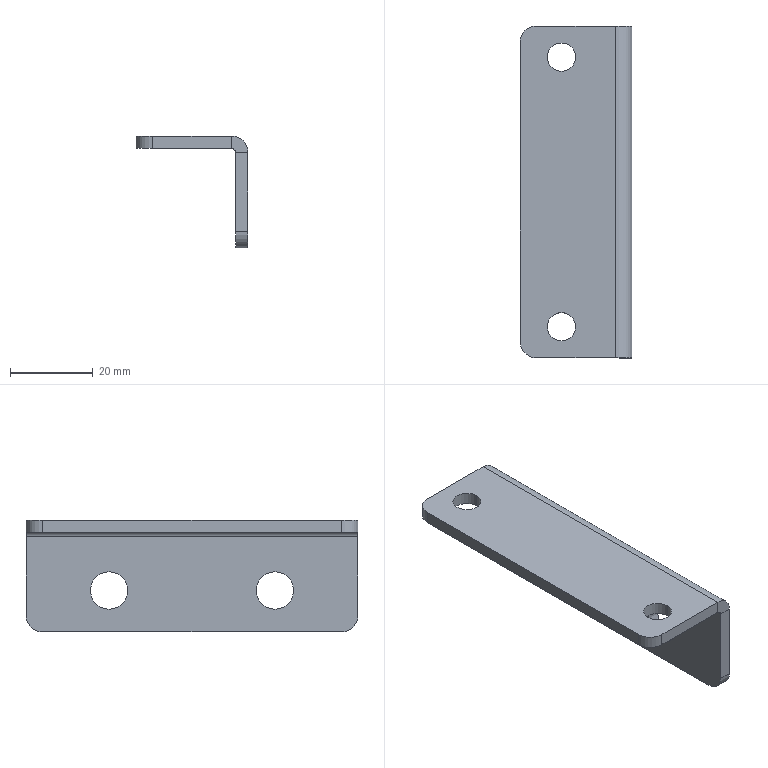Part | STEP file | 1.6米L型片 | 1 solid | 26 faces | box 27 x 80 x 27 mm | volume 11342 mm3 | cylinder 14 | plane 12 | commonest cylinder face diameters 8 x5 6.8 x4 9 x4 2 x1
STEP:
#1=CARTESIAN_POINT('',(27.,20.,-21.5));
#2=VERTEX_POINT('',#1);
#3=CARTESIAN_POINT('',(27.,20.,-12.5));
#4=VERTEX_POINT('',#3);
#5=CARTESIAN_POINT('',(27.,20.,-17.));
#6=DIRECTION('',(-1.,0.,0.));
#7=DIRECTION('',(0.,0.,1.));
#8=AXIS2_PLACEMENT_3D('',#5,#6,#7);
#9=CIRCLE('',#8,4.5);
#10=EDGE_CURVE('',#2,#4,#9,.T.);
#11=ORIENTED_EDGE('',*,*,#10,.F.);
#12=CARTESIAN_POINT('',(24.,20.,-21.5));
#13=VERTEX_POINT('',#12);
#14=CARTESIAN_POINT('',(34.,20.,-21.5));
#15=DIRECTION('',(-1.,0.,0.));
#16=VECTOR('',#15,1000.);
#17=LINE('',#14,#16);
#18=EDGE_CURVE('',#2,#13,#17,.T.);
#19=ORIENTED_EDGE('',*,*,#18,.T.);
#20=CARTESIAN_POINT('',(24.,20.,-12.5));
#21=VERTEX_POINT('',#20);
#22=CARTESIAN_POINT('',(24.,20.,-17.));
#23=DIRECTION('',(-1.,0.,0.));
#24=DIRECTION('',(0.,0.,1.));
#25=AXIS2_PLACEMENT_3D('',#22,#23,#24);
#26=CIRCLE('',#25,4.5);
#27=EDGE_CURVE('',#13,#21,#26,.T.);
#28=ORIENTED_EDGE('',*,*,#27,.T.);
#29=CARTESIAN_POINT('',(34.,20.,-12.5));
#30=DIRECTION('',(-1.,0.,0.));
#31=VECTOR('',#30,1000.);
#32=LINE('',#29,#31);
#33=EDGE_CURVE('',#4,#21,#32,.T.);
#34=ORIENTED_EDGE('',*,*,#33,.F.);
#35=EDGE_LOOP('',(#11,#19,#28,#34));
#36=FACE_OUTER_BOUND('',#35,.T.);
#37=CARTESIAN_POINT('',(34.,20.,-17.));
#38=DIRECTION('',(-1.,0.,0.));
#39=DIRECTION('',(0.,0.,1.));
#40=AXIS2_PLACEMENT_3D('',#37,#38,#39);
#41=CYLINDRICAL_SURFACE('',#40,4.5);
#42=ADVANCED_FACE('',(#36),#41,.F.);
#43=CARTESIAN_POINT('',(27.,60.,-21.5));
#44=VERTEX_POINT('',#43);
#45=CARTESIAN_POINT('',(27.,60.,-12.5));
#46=VERTEX_POINT('',#45);
#47=CARTESIAN_POINT('',(27.,60.,-17.));
#48=DIRECTION('',(-1.,0.,0.));
#49=DIRECTION('',(0.,0.,1.));
#50=AXIS2_PLACEMENT_3D('',#47,#48,#49);
#51=CIRCLE('',#50,4.5);
#52=EDGE_CURVE('',#44,#46,#51,.T.);
#53=ORIENTED_EDGE('',*,*,#52,.F.);
#54=CARTESIAN_POINT('',(24.,60.,-21.5));
#55=VERTEX_POINT('',#54);
#56=CARTESIAN_POINT('',(34.,60.,-21.5));
#57=DIRECTION('',(-1.,0.,0.));
#58=VECTOR('',#57,1000.);
#59=LINE('',#56,#58);
#60=EDGE_CURVE('',#44,#55,#59,.T.);
#61=ORIENTED_EDGE('',*,*,#60,.T.);
#62=CARTESIAN_POINT('',(24.,60.,-12.5));
#63=VERTEX_POINT('',#62);
#64=CARTESIAN_POINT('',(24.,60.,-17.));
#65=DIRECTION('',(-1.,0.,0.));
#66=DIRECTION('',(0.,0.,1.));
#67=AXIS2_PLACEMENT_3D('',#64,#65,#66);
#68=CIRCLE('',#67,4.5);
#69=EDGE_CURVE('',#55,#63,#68,.T.);
#70=ORIENTED_EDGE('',*,*,#69,.T.);
#71=CARTESIAN_POINT('',(34.,60.,-12.5));
#72=DIRECTION('',(-1.,0.,0.));
#73=VECTOR('',#72,1000.);
#74=LINE('',#71,#73);
#75=EDGE_CURVE('',#46,#63,#74,.T.);
#76=ORIENTED_EDGE('',*,*,#75,.F.);
#77=EDGE_LOOP('',(#53,#61,#70,#76));
#78=FACE_OUTER_BOUND('',#77,.T.);
#79=CARTESIAN_POINT('',(34.,60.,-17.));
#80=DIRECTION('',(-1.,0.,0.));
#81=DIRECTION('',(0.,0.,1.));
#82=AXIS2_PLACEMENT_3D('',#79,#80,#81);
#83=CYLINDRICAL_SURFACE('',#82,4.5);
#84=ADVANCED_FACE('',(#78),#83,.F.);
#85=CARTESIAN_POINT('',(13.4,72.5,0.));
#86=VERTEX_POINT('',#85);
#87=CARTESIAN_POINT('',(6.6,72.5,0.));
#88=VERTEX_POINT('',#87);
#89=CARTESIAN_POINT('',(10.,72.5,0.));
#90=DIRECTION('',(0.,0.,-1.));
#91=DIRECTION('',(-1.,0.,0.));
#92=AXIS2_PLACEMENT_3D('',#89,#90,#91);
#93=CIRCLE('',#92,3.4);
#94=EDGE_CURVE('',#86,#88,#93,.T.);
#95=ORIENTED_EDGE('',*,*,#94,.F.);
#96=CARTESIAN_POINT('',(13.4,72.5,-3.));
#97=VERTEX_POINT('',#96);
#98=CARTESIAN_POINT('',(13.4,72.5,-3.));
#99=DIRECTION('',(0.,0.,-1.));
#100=VECTOR('',#99,1000.);
#101=LINE('',#98,#100);
#102=EDGE_CURVE('',#86,#97,#101,.T.);
#103=ORIENTED_EDGE('',*,*,#102,.T.);
#104=CARTESIAN_POINT('',(6.6,72.5,-3.));
#105=VERTEX_POINT('',#104);
#106=CARTESIAN_POINT('',(10.,72.5,-3.));
#107=DIRECTION('',(0.,0.,-1.));
#108=DIRECTION('',(-1.,0.,0.));
#109=AXIS2_PLACEMENT_3D('',#106,#107,#108);
#110=CIRCLE('',#109,3.4);
#111=EDGE_CURVE('',#97,#105,#110,.T.);
#112=ORIENTED_EDGE('',*,*,#111,.T.);
#113=CARTESIAN_POINT('',(6.6,72.5,-3.));
#114=DIRECTION('',(0.,0.,-1.));
#115=VECTOR('',#114,1000.);
#116=LINE('',#113,#115);
#117=EDGE_CURVE('',#88,#105,#116,.T.);
#118=ORIENTED_EDGE('',*,*,#117,.F.);
#119=EDGE_LOOP('',(#95,#103,#112,#118));
#120=FACE_OUTER_BOUND('',#119,.T.);
#121=CARTESIAN_POINT('',(10.,72.5,-3.));
#122=DIRECTION('',(0.,0.,-1.));
#123=DIRECTION('',(-1.,0.,0.));
#124=AXIS2_PLACEMENT_3D('',#121,#122,#123);
#125=CYLINDRICAL_SURFACE('',#124,3.4);
#126=ADVANCED_FACE('',(#120),#125,.F.);
#127=CARTESIAN_POINT('',(13.4,7.5,0.));
#128=VERTEX_POINT('',#127);
#129=CARTESIAN_POINT('',(6.6,7.5,0.));
#130=VERTEX_POINT('',#129);
#131=CARTESIAN_POINT('',(10.,7.5,0.));
#132=DIRECTION('',(0.,0.,-1.));
#133=DIRECTION('',(-1.,0.,0.));
#134=AXIS2_PLACEMENT_3D('',#131,#132,#133);
#135=CIRCLE('',#134,3.4);
#136=EDGE_CURVE('',#128,#130,#135,.T.);
#137=ORIENTED_EDGE('',*,*,#136,.F.);
#138=CARTESIAN_POINT('',(13.4,7.5,-3.));
#139=VERTEX_POINT('',#138);
#140=CARTESIAN_POINT('',(13.4,7.5,-3.));
#141=DIRECTION('',(0.,0.,-1.));
#142=VECTOR('',#141,1000.);
#143=LINE('',#140,#142);
#144=EDGE_CURVE('',#128,#139,#143,.T.);
#145=ORIENTED_EDGE('',*,*,#144,.T.);
#146=CARTESIAN_POINT('',(6.6,7.5,-3.));
#147=VERTEX_POINT('',#146);
#148=CARTESIAN_POINT('',(10.,7.5,-3.));
#149=DIRECTION('',(0.,0.,-1.));
#150=DIRECTION('',(-1.,0.,0.));
#151=AXIS2_PLACEMENT_3D('',#148,#149,#150);
#152=CIRCLE('',#151,3.4);
#153=EDGE_CURVE('',#139,#147,#152,.T.);
#154=ORIENTED_EDGE('',*,*,#153,.T.);
#155=CARTESIAN_POINT('',(6.6,7.5,-3.));
#156=DIRECTION('',(0.,0.,-1.));
#157=VECTOR('',#156,1000.);
#158=LINE('',#155,#157);
#159=EDGE_CURVE('',#130,#147,#158,.T.);
#160=ORIENTED_EDGE('',*,*,#159,.F.);
#161=EDGE_LOOP('',(#137,#145,#154,#160));
#162=FACE_OUTER_BOUND('',#161,.T.);
#163=CARTESIAN_POINT('',(10.,7.5,-3.));
#164=DIRECTION('',(0.,0.,-1.));
#165=DIRECTION('',(-1.,0.,0.));
#166=AXIS2_PLACEMENT_3D('',#163,#164,#165);
#167=CYLINDRICAL_SURFACE('',#166,3.4);
#168=ADVANCED_FACE('',(#162),#167,.F.);
#169=CARTESIAN_POINT('',(23.,80.,0.));
#170=VERTEX_POINT('',#169);
#171=CARTESIAN_POINT('',(23.,80.,-3.));
#172=VERTEX_POINT('',#171);
#173=CARTESIAN_POINT('',(23.,80.,0.));
#174=DIRECTION('',(0.,0.,-1.));
#175=VECTOR('',#174,1000.);
#176=LINE('',#173,#175);
#177=EDGE_CURVE('',#170,#172,#176,.T.);
#178=ORIENTED_EDGE('',*,*,#177,.F.);
#179=CARTESIAN_POINT('',(27.,80.,-4.));
#180=VERTEX_POINT('',#179);
#181=CARTESIAN_POINT('',(23.,80.,-4.));
#182=DIRECTION('',(0.,1.,0.));
#183=DIRECTION('',(0.,0.,-1.));
#184=AXIS2_PLACEMENT_3D('',#181,#182,#183);
#185=CIRCLE('',#184,4.);
#186=EDGE_CURVE('',#170,#180,#185,.T.);
#187=ORIENTED_EDGE('',*,*,#186,.T.);
#188=CARTESIAN_POINT('',(24.,80.,-4.));
#189=VERTEX_POINT('',#188);
#190=CARTESIAN_POINT('',(24.,80.,-4.));
#191=DIRECTION('',(1.,0.,0.));
#192=VECTOR('',#191,1000.);
#193=LINE('',#190,#192);
#194=EDGE_CURVE('',#189,#180,#193,.T.);
#195=ORIENTED_EDGE('',*,*,#194,.F.);
#196=CARTESIAN_POINT('',(23.,80.,-4.));
#197=DIRECTION('',(0.,1.,0.));
#198=DIRECTION('',(1.,0.,0.));
#199=AXIS2_PLACEMENT_3D('',#196,#197,#198);
#200=CIRCLE('',#199,1.);
#201=EDGE_CURVE('',#172,#189,#200,.T.);
#202=ORIENTED_EDGE('',*,*,#201,.F.);
#203=EDGE_LOOP('',(#178,#187,#195,#202));
#204=FACE_OUTER_BOUND('',#203,.T.);
#205=CARTESIAN_POINT('',(23.,80.,0.));
#206=DIRECTION('',(0.,1.,0.));
#207=DIRECTION('',(0.,0.,1.));
#208=AXIS2_PLACEMENT_3D('',#205,#206,#207);
#209=PLANE('',#208);
#210=ADVANCED_FACE('',(#204),#209,.T.);
#211=CARTESIAN_POINT('',(4.,80.,-3.));
#212=VERTEX_POINT('',#211);
#213=CARTESIAN_POINT('',(0.,80.,-3.));
#214=DIRECTION('',(1.,0.,0.));
#215=VECTOR('',#214,1000.);
#216=LINE('',#213,#215);
#217=EDGE_CURVE('',#212,#172,#216,.T.);
#218=ORIENTED_EDGE('',*,*,#217,.F.);
#219=CARTESIAN_POINT('',(4.,80.,0.));
#220=VERTEX_POINT('',#219);
#221=CARTESIAN_POINT('',(4.,80.,-4.));
#222=DIRECTION('',(0.,0.,1.));
#223=VECTOR('',#222,1000.);
#224=LINE('',#221,#223);
#225=EDGE_CURVE('',#212,#220,#224,.T.);
#226=ORIENTED_EDGE('',*,*,#225,.T.);
#227=CARTESIAN_POINT('',(0.,80.,0.));
#228=DIRECTION('',(1.,0.,0.));
#229=VECTOR('',#228,1000.);
#230=LINE('',#227,#229);
#231=EDGE_CURVE('',#220,#170,#230,.T.);
#232=ORIENTED_EDGE('',*,*,#231,.T.);
#233=ORIENTED_EDGE('',*,*,#177,.T.);
#234=EDGE_LOOP('',(#218,#226,#232,#233));
#235=FACE_OUTER_BOUND('',#234,.T.);
#236=CARTESIAN_POINT('',(24.,80.,-4.));
#237=DIRECTION('',(0.,1.,0.));
#238=DIRECTION('',(0.,0.,1.));
#239=AXIS2_PLACEMENT_3D('',#236,#237,#238);
#240=PLANE('',#239);
#241=ADVANCED_FACE('',(#235),#240,.T.);
#242=CARTESIAN_POINT('',(27.,0.,-4.));
#243=VERTEX_POINT('',#242);
#244=CARTESIAN_POINT('',(24.,0.,-4.));
#245=VERTEX_POINT('',#244);
#246=CARTESIAN_POINT('',(27.,0.,-4.));
#247=DIRECTION('',(-1.,0.,0.));
#248=VECTOR('',#247,1000.);
#249=LINE('',#246,#248);
#250=EDGE_CURVE('',#243,#245,#249,.T.);
#251=ORIENTED_EDGE('',*,*,#250,.F.);
#252=CARTESIAN_POINT('',(23.,0.,0.));
#253=VERTEX_POINT('',#252);
#254=CARTESIAN_POINT('',(23.,0.,-4.));
#255=DIRECTION('',(0.,1.,0.));
#256=DIRECTION('',(0.,0.,-1.));
#257=AXIS2_PLACEMENT_3D('',#254,#255,#256);
#258=CIRCLE('',#257,4.);
#259=EDGE_CURVE('',#253,#243,#258,.T.);
#260=ORIENTED_EDGE('',*,*,#259,.F.);
#261=CARTESIAN_POINT('',(23.,0.,-3.));
#262=VERTEX_POINT('',#261);
#263=CARTESIAN_POINT('',(23.,0.,-3.));
#264=DIRECTION('',(0.,0.,1.));
#265=VECTOR('',#264,1000.);
#266=LINE('',#263,#265);
#267=EDGE_CURVE('',#262,#253,#266,.T.);
#268=ORIENTED_EDGE('',*,*,#267,.F.);
#269=CARTESIAN_POINT('',(23.,0.,-4.));
#270=DIRECTION('',(0.,1.,0.));
#271=DIRECTION('',(1.,0.,0.));
#272=AXIS2_PLACEMENT_3D('',#269,#270,#271);
#273=CIRCLE('',#272,1.);
#274=EDGE_CURVE('',#262,#245,#273,.T.);
#275=ORIENTED_EDGE('',*,*,#274,.T.);
#276=EDGE_LOOP('',(#251,#260,#268,#275));
#277=FACE_OUTER_BOUND('',#276,.T.);
#278=CARTESIAN_POINT('',(27.,0.,-4.));
#279=DIRECTION('',(0.,-1.,0.));
#280=DIRECTION('',(0.,0.,-1.));
#281=AXIS2_PLACEMENT_3D('',#278,#279,#280);
#282=PLANE('',#281);
#283=ADVANCED_FACE('',(#277),#282,.T.);
#284=CARTESIAN_POINT('',(24.,0.,-23.));
#285=VERTEX_POINT('',#284);
#286=CARTESIAN_POINT('',(24.,0.,0.));
#287=DIRECTION('',(0.,0.,-1.));
#288=VECTOR('',#287,1000.);
#289=LINE('',#286,#288);
#290=EDGE_CURVE('',#245,#285,#289,.T.);
#291=ORIENTED_EDGE('',*,*,#290,.T.);
#292=CARTESIAN_POINT('',(27.,0.,-23.));
#293=VERTEX_POINT('',#292);
#294=CARTESIAN_POINT('',(23.,0.,-23.));
#295=DIRECTION('',(1.,0.,0.));
#296=VECTOR('',#295,1000.);
#297=LINE('',#294,#296);
#298=EDGE_CURVE('',#285,#293,#297,.T.);
#299=ORIENTED_EDGE('',*,*,#298,.T.);
#300=CARTESIAN_POINT('',(27.,0.,0.));
#301=DIRECTION('',(0.,0.,-1.));
#302=VECTOR('',#301,1000.);
#303=LINE('',#300,#302);
#304=EDGE_CURVE('',#243,#293,#303,.T.);
#305=ORIENTED_EDGE('',*,*,#304,.F.);
#306=ORIENTED_EDGE('',*,*,#250,.T.);
#307=EDGE_LOOP('',(#291,#299,#305,#306));
#308=FACE_OUTER_BOUND('',#307,.T.);
#309=CARTESIAN_POINT('',(23.,0.,-3.));
#310=DIRECTION('',(0.,-1.,0.));
#311=DIRECTION('',(0.,0.,-1.));
#312=AXIS2_PLACEMENT_3D('',#309,#310,#311);
#313=PLANE('',#312);
#314=ADVANCED_FACE('',(#308),#313,.T.);
#315=CARTESIAN_POINT('',(27.,20.,-17.));
#316=DIRECTION('',(-1.,0.,0.));
#317=DIRECTION('',(0.,0.,1.));
#318=AXIS2_PLACEMENT_3D('',#315,#316,#317);
#319=CIRCLE('',#318,4.5);
#320=EDGE_CURVE('',#4,#2,#319,.T.);
#321=ORIENTED_EDGE('',*,*,#320,.T.);
#322=ORIENTED_EDGE('',*,*,#10,.T.);
#323=EDGE_LOOP('',(#321,#322));
#324=FACE_BOUND('',#323,.T.);
#325=CARTESIAN_POINT('',(27.,60.,-17.));
#326=DIRECTION('',(-1.,0.,0.));
#327=DIRECTION('',(0.,0.,1.));
#328=AXIS2_PLACEMENT_3D('',#325,#326,#327);
#329=CIRCLE('',#328,4.5);
#330=EDGE_CURVE('',#46,#44,#329,.T.);
#331=ORIENTED_EDGE('',*,*,#330,.T.);
#332=ORIENTED_EDGE('',*,*,#52,.T.);
#333=EDGE_LOOP('',(#331,#332));
#334=FACE_BOUND('',#333,.T.);
#335=CARTESIAN_POINT('',(27.,76.,-27.));
#336=VERTEX_POINT('',#335);
#337=CARTESIAN_POINT('',(27.,4.,-27.));
#338=VERTEX_POINT('',#337);
#339=CARTESIAN_POINT('',(27.,80.,-27.));
#340=DIRECTION('',(0.,-1.,0.));
#341=VECTOR('',#340,1000.);
#342=LINE('',#339,#341);
#343=EDGE_CURVE('',#336,#338,#342,.T.);
#344=ORIENTED_EDGE('',*,*,#343,.F.);
#345=CARTESIAN_POINT('',(27.,80.,-23.));
#346=VERTEX_POINT('',#345);
#347=CARTESIAN_POINT('',(27.,76.,-23.));
#348=DIRECTION('',(1.,0.,0.));
#349=DIRECTION('',(0.,0.,1.));
#350=AXIS2_PLACEMENT_3D('',#347,#348,#349);
#351=CIRCLE('',#350,4.);
#352=EDGE_CURVE('',#336,#346,#351,.T.);
#353=ORIENTED_EDGE('',*,*,#352,.T.);
#354=CARTESIAN_POINT('',(27.,80.,0.));
#355=DIRECTION('',(0.,0.,-1.));
#356=VECTOR('',#355,1000.);
#357=LINE('',#354,#356);
#358=EDGE_CURVE('',#180,#346,#357,.T.);
#359=ORIENTED_EDGE('',*,*,#358,.F.);
#360=CARTESIAN_POINT('',(27.,80.,-4.));
#361=DIRECTION('',(0.,-1.,0.));
#362=VECTOR('',#361,1000.);
#363=LINE('',#360,#362);
#364=EDGE_CURVE('',#180,#243,#363,.T.);
#365=ORIENTED_EDGE('',*,*,#364,.T.);
#366=ORIENTED_EDGE('',*,*,#304,.T.);
#367=CARTESIAN_POINT('',(27.,4.,-23.));
#368=DIRECTION('',(1.,0.,0.));
#369=DIRECTION('',(0.,0.,1.));
#370=AXIS2_PLACEMENT_3D('',#367,#368,#369);
#371=CIRCLE('',#370,4.);
#372=EDGE_CURVE('',#293,#338,#371,.T.);
#373=ORIENTED_EDGE('',*,*,#372,.T.);
#374=EDGE_LOOP('',(#344,#353,#359,#365,#366,#373));
#375=FACE_OUTER_BOUND('',#374,.T.);
#376=CARTESIAN_POINT('',(27.,80.,0.));
#377=DIRECTION('',(-1.,0.,0.));
#378=DIRECTION('',(0.,0.,1.));
#379=AXIS2_PLACEMENT_3D('',#376,#377,#378);
#380=PLANE('',#379);
#381=ADVANCED_FACE('',(#324,#334,#375),#380,.F.);
#382=CARTESIAN_POINT('',(24.,76.,-27.));
#383=VERTEX_POINT('',#382);
#384=CARTESIAN_POINT('',(24.,4.,-27.));
#385=VERTEX_POINT('',#384);
#386=CARTESIAN_POINT('',(24.,80.,-27.));
#387=DIRECTION('',(0.,-1.,0.));
#388=VECTOR('',#387,1000.);
#389=LINE('',#386,#388);
#390=EDGE_CURVE('',#383,#385,#389,.T.);
#391=ORIENTED_EDGE('',*,*,#390,.F.);
#392=CARTESIAN_POINT('',(24.,76.,-27.));
#393=DIRECTION('',(1.,0.,0.));
#394=VECTOR('',#393,1000.);
#395=LINE('',#392,#394);
#396=EDGE_CURVE('',#383,#336,#395,.T.);
#397=ORIENTED_EDGE('',*,*,#396,.T.);
#398=ORIENTED_EDGE('',*,*,#343,.T.);
#399=CARTESIAN_POINT('',(24.,4.,-27.));
#400=DIRECTION('',(-1.,0.,0.));
#401=VECTOR('',#400,1000.);
#402=LINE('',#399,#401);
#403=EDGE_CURVE('',#338,#385,#402,.T.);
#404=ORIENTED_EDGE('',*,*,#403,.T.);
#405=EDGE_LOOP('',(#391,#397,#398,#404));
#406=FACE_OUTER_BOUND('',#405,.T.);
#407=CARTESIAN_POINT('',(24.,80.,-27.));
#408=DIRECTION('',(0.,0.,-1.));
#409=DIRECTION('',(-1.,0.,0.));
#410=AXIS2_PLACEMENT_3D('',#407,#408,#409);
#411=PLANE('',#410);
#412=ADVANCED_FACE('',(#406),#411,.T.);
#413=CARTESIAN_POINT('',(24.,20.,-17.));
#414=DIRECTION('',(-1.,0.,0.));
#415=DIRECTION('',(0.,0.,1.));
#416=AXIS2_PLACEMENT_3D('',#413,#414,#415);
#417=CIRCLE('',#416,4.5);
#418=EDGE_CURVE('',#21,#13,#417,.T.);
#419=ORIENTED_EDGE('',*,*,#418,.F.);
#420=ORIENTED_EDGE('',*,*,#27,.F.);
#421=EDGE_LOOP('',(#419,#420));
#422=FACE_BOUND('',#421,.T.);
#423=CARTESIAN_POINT('',(24.,60.,-17.));
#424=DIRECTION('',(-1.,0.,0.));
#425=DIRECTION('',(0.,0.,1.));
#426=AXIS2_PLACEMENT_3D('',#423,#424,#425);
#427=CIRCLE('',#426,4.5);
#428=EDGE_CURVE('',#63,#55,#427,.T.);
#429=ORIENTED_EDGE('',*,*,#428,.F.);
#430=ORIENTED_EDGE('',*,*,#69,.F.);
#431=EDGE_LOOP('',(#429,#430));
#432=FACE_BOUND('',#431,.T.);
#433=CARTESIAN_POINT('',(24.,80.,-23.));
#434=VERTEX_POINT('',#433);
#435=CARTESIAN_POINT('',(24.,80.,0.));
#436=DIRECTION('',(0.,0.,-1.));
#437=VECTOR('',#436,1000.);
#438=LINE('',#435,#437);
#439=EDGE_CURVE('',#189,#434,#438,.T.);
#440=ORIENTED_EDGE('',*,*,#439,.T.);
#441=CARTESIAN_POINT('',(24.,76.,-23.));
#442=DIRECTION('',(-1.,0.,0.));
#443=DIRECTION('',(0.,0.,1.));
#444=AXIS2_PLACEMENT_3D('',#441,#442,#443);
#445=CIRCLE('',#444,4.);
#446=EDGE_CURVE('',#434,#383,#445,.T.);
#447=ORIENTED_EDGE('',*,*,#446,.T.);
#448=ORIENTED_EDGE('',*,*,#390,.T.);
#449=CARTESIAN_POINT('',(24.,4.,-23.));
#450=DIRECTION('',(-1.,0.,0.));
#451=DIRECTION('',(0.,0.,1.));
#452=AXIS2_PLACEMENT_3D('',#449,#450,#451);
#453=CIRCLE('',#452,4.);
#454=EDGE_CURVE('',#385,#285,#453,.T.);
#455=ORIENTED_EDGE('',*,*,#454,.T.);
#456=ORIENTED_EDGE('',*,*,#290,.F.);
#457=CARTESIAN_POINT('',(24.,80.,-4.));
#458=DIRECTION('',(0.,-1.,0.));
#459=VECTOR('',#458,1000.);
#460=LINE('',#457,#459);
#461=EDGE_CURVE('',#189,#245,#460,.T.);
#462=ORIENTED_EDGE('',*,*,#461,.F.);
#463=EDGE_LOOP('',(#440,#447,#448,#455,#456,#462));
#464=FACE_OUTER_BOUND('',#463,.T.);
#465=CARTESIAN_POINT('',(24.,80.,0.));
#466=DIRECTION('',(-1.,0.,0.));
#467=DIRECTION('',(0.,0.,1.));
#468=AXIS2_PLACEMENT_3D('',#465,#466,#467);
#469=PLANE('',#468);
#470=ADVANCED_FACE('',(#422,#432,#464),#469,.T.);
#471=ORIENTED_EDGE('',*,*,#274,.F.);
#472=CARTESIAN_POINT('',(23.,80.,-3.));
#473=DIRECTION('',(0.,-1.,0.));
#474=VECTOR('',#473,1000.);
#475=LINE('',#472,#474);
#476=EDGE_CURVE('',#172,#262,#475,.T.);
#477=ORIENTED_EDGE('',*,*,#476,.F.);
#478=ORIENTED_EDGE('',*,*,#201,.T.);
#479=ORIENTED_EDGE('',*,*,#461,.T.);
#480=EDGE_LOOP('',(#471,#477,#478,#479));
#481=FACE_OUTER_BOUND('',#480,.T.);
#482=CARTESIAN_POINT('',(23.,80.,-4.));
#483=DIRECTION('',(0.,-1.,0.));
#484=DIRECTION('',(0.,0.,-1.));
#485=AXIS2_PLACEMENT_3D('',#482,#483,#484);
#486=CYLINDRICAL_SURFACE('',#485,1.);
#487=ADVANCED_FACE('',(#481),#486,.F.);
#488=CARTESIAN_POINT('',(10.,72.5,-3.));
#489=DIRECTION('',(0.,0.,-1.));
#490=DIRECTION('',(-1.,0.,0.));
#491=AXIS2_PLACEMENT_3D('',#488,#489,#490);
#492=CIRCLE('',#491,3.4);
#493=EDGE_CURVE('',#105,#97,#492,.T.);
#494=ORIENTED_EDGE('',*,*,#493,.F.);
#495=ORIENTED_EDGE('',*,*,#111,.F.);
#496=EDGE_LOOP('',(#494,#495));
#497=FACE_BOUND('',#496,.T.);
#498=CARTESIAN_POINT('',(10.,7.5,-3.));
#499=DIRECTION('',(0.,0.,-1.));
#500=DIRECTION('',(-1.,0.,0.));
#501=AXIS2_PLACEMENT_3D('',#498,#499,#500);
#502=CIRCLE('',#501,3.4);
#503=EDGE_CURVE('',#147,#139,#502,.T.);
#504=ORIENTED_EDGE('',*,*,#503,.F.);
#505=ORIENTED_EDGE('',*,*,#153,.F.);
#506=EDGE_LOOP('',(#504,#505));
#507=FACE_BOUND('',#506,.T.);
#508=CARTESIAN_POINT('',(4.,0.,-3.));
#509=VERTEX_POINT('',#508);
#510=CARTESIAN_POINT('',(0.,0.,-3.));
#511=DIRECTION('',(1.,0.,0.));
#512=VECTOR('',#511,1000.);
#513=LINE('',#510,#512);
#514=EDGE_CURVE('',#509,#262,#513,.T.);
#515=ORIENTED_EDGE('',*,*,#514,.F.);
#516=CARTESIAN_POINT('',(0.,4.,-3.));
#517=VERTEX_POINT('',#516);
#518=CARTESIAN_POINT('',(4.,4.,-3.));
#519=DIRECTION('',(0.,0.,-1.));
#520=DIRECTION('',(-1.,0.,0.));
#521=AXIS2_PLACEMENT_3D('',#518,#519,#520);
#522=CIRCLE('',#521,4.);
#523=EDGE_CURVE('',#509,#517,#522,.T.);
#524=ORIENTED_EDGE('',*,*,#523,.T.);
#525=CARTESIAN_POINT('',(0.,76.,-3.));
#526=VERTEX_POINT('',#525);
#527=CARTESIAN_POINT('',(0.,80.,-3.));
#528=DIRECTION('',(0.,-1.,0.));
#529=VECTOR('',#528,1000.);
#530=LINE('',#527,#529);
#531=EDGE_CURVE('',#526,#517,#530,.T.);
#532=ORIENTED_EDGE('',*,*,#531,.F.);
#533=CARTESIAN_POINT('',(4.,76.,-3.));
#534=DIRECTION('',(0.,0.,-1.));
#535=DIRECTION('',(-1.,0.,0.));
#536=AXIS2_PLACEMENT_3D('',#533,#534,#535);
#537=CIRCLE('',#536,4.);
#538=EDGE_CURVE('',#526,#212,#537,.T.);
#539=ORIENTED_EDGE('',*,*,#538,.T.);
#540=ORIENTED_EDGE('',*,*,#217,.T.);
#541=ORIENTED_EDGE('',*,*,#476,.T.);
#542=EDGE_LOOP('',(#515,#524,#532,#539,#540,#541));
#543=FACE_OUTER_BOUND('',#542,.T.);
#544=CARTESIAN_POINT('',(0.,80.,-3.));
#545=DIRECTION('',(0.,0.,-1.));
#546=DIRECTION('',(-1.,0.,0.));
#547=AXIS2_PLACEMENT_3D('',#544,#545,#546);
#548=PLANE('',#547);
#549=ADVANCED_FACE('',(#497,#507,#543),#548,.T.);
#550=ORIENTED_EDGE('',*,*,#531,.T.);
#551=CARTESIAN_POINT('',(0.,4.,0.));
#552=VERTEX_POINT('',#551);
#553=CARTESIAN_POINT('',(0.,4.,0.));
#554=DIRECTION('',(0.,0.,1.));
#555=VECTOR('',#554,1000.);
#556=LINE('',#553,#555);
#557=EDGE_CURVE('',#517,#552,#556,.T.);
#558=ORIENTED_EDGE('',*,*,#557,.T.);
#559=CARTESIAN_POINT('',(0.,76.,0.));
#560=VERTEX_POINT('',#559);
#561=CARTESIAN_POINT('',(0.,80.,0.));
#562=DIRECTION('',(0.,-1.,0.));
#563=VECTOR('',#562,1000.);
#564=LINE('',#561,#563);
#565=EDGE_CURVE('',#560,#552,#564,.T.);
#566=ORIENTED_EDGE('',*,*,#565,.F.);
#567=CARTESIAN_POINT('',(0.,76.,0.));
#568=DIRECTION('',(0.,0.,-1.));
#569=VECTOR('',#568,1000.);
#570=LINE('',#567,#569);
#571=EDGE_CURVE('',#560,#526,#570,.T.);
#572=ORIENTED_EDGE('',*,*,#571,.T.);
#573=EDGE_LOOP('',(#550,#558,#566,#572));
#574=FACE_OUTER_BOUND('',#573,.T.);
#575=CARTESIAN_POINT('',(0.,80.,0.));
#576=DIRECTION('',(-1.,0.,0.));
#577=DIRECTION('',(0.,0.,1.));
#578=AXIS2_PLACEMENT_3D('',#575,#576,#577);
#579=PLANE('',#578);
#580=ADVANCED_FACE('',(#574),#579,.T.);
#581=CARTESIAN_POINT('',(10.,72.5,0.));
#582=DIRECTION('',(0.,0.,-1.));
#583=DIRECTION('',(-1.,0.,0.));
#584=AXIS2_PLACEMENT_3D('',#581,#582,#583);
#585=CIRCLE('',#584,3.4);
#586=EDGE_CURVE('',#88,#86,#585,.T.);
#587=ORIENTED_EDGE('',*,*,#586,.T.);
#588=ORIENTED_EDGE('',*,*,#94,.T.);
#589=EDGE_LOOP('',(#587,#588));
#590=FACE_BOUND('',#589,.T.);
#591=CARTESIAN_POINT('',(10.,7.5,0.));
#592=DIRECTION('',(0.,0.,-1.));
#593=DIRECTION('',(-1.,0.,0.));
#594=AXIS2_PLACEMENT_3D('',#591,#592,#593);
#595=CIRCLE('',#594,3.4);
#596=EDGE_CURVE('',#130,#128,#595,.T.);
#597=ORIENTED_EDGE('',*,*,#596,.T.);
#598=ORIENTED_EDGE('',*,*,#136,.T.);
#599=EDGE_LOOP('',(#597,#598));
#600=FACE_BOUND('',#599,.T.);
#601=ORIENTED_EDGE('',*,*,#565,.T.);
#602=CARTESIAN_POINT('',(4.,0.,0.));
#603=VERTEX_POINT('',#602);
#604=CARTESIAN_POINT('',(4.,4.,0.));
#605=DIRECTION('',(0.,0.,1.));
#606=DIRECTION('',(-1.,0.,0.));
#607=AXIS2_PLACEMENT_3D('',#604,#605,#606);
#608=CIRCLE('',#607,4.);
#609=EDGE_CURVE('',#552,#603,#608,.T.);
#610=ORIENTED_EDGE('',*,*,#609,.T.);
#611=CARTESIAN_POINT('',(0.,0.,0.));
#612=DIRECTION('',(1.,0.,0.));
#613=VECTOR('',#612,1000.);
#614=LINE('',#611,#613);
#615=EDGE_CURVE('',#603,#253,#614,.T.);
#616=ORIENTED_EDGE('',*,*,#615,.T.);
#617=CARTESIAN_POINT('',(23.,80.,0.));
#618=DIRECTION('',(0.,-1.,0.));
#619=VECTOR('',#618,1000.);
#620=LINE('',#617,#619);
#621=EDGE_CURVE('',#170,#253,#620,.T.);
#622=ORIENTED_EDGE('',*,*,#621,.F.);
#623=ORIENTED_EDGE('',*,*,#231,.F.);
#624=CARTESIAN_POINT('',(4.,76.,0.));
#625=DIRECTION('',(0.,0.,1.));
#626=DIRECTION('',(-1.,0.,0.));
#627=AXIS2_PLACEMENT_3D('',#624,#625,#626);
#628=CIRCLE('',#627,4.);
#629=EDGE_CURVE('',#220,#560,#628,.T.);
#630=ORIENTED_EDGE('',*,*,#629,.T.);
#631=EDGE_LOOP('',(#601,#610,#616,#622,#623,#630));
#632=FACE_OUTER_BOUND('',#631,.T.);
#633=CARTESIAN_POINT('',(0.,80.,0.));
#634=DIRECTION('',(0.,0.,-1.));
#635=DIRECTION('',(-1.,0.,0.));
#636=AXIS2_PLACEMENT_3D('',#633,#634,#635);
#637=PLANE('',#636);
#638=ADVANCED_FACE('',(#590,#600,#632),#637,.F.);
#639=ORIENTED_EDGE('',*,*,#259,.T.);
#640=ORIENTED_EDGE('',*,*,#364,.F.);
#641=ORIENTED_EDGE('',*,*,#186,.F.);
#642=ORIENTED_EDGE('',*,*,#621,.T.);
#643=EDGE_LOOP('',(#639,#640,#641,#642));
#644=FACE_OUTER_BOUND('',#643,.T.);
#645=CARTESIAN_POINT('',(23.,80.,-4.));
#646=DIRECTION('',(0.,-1.,0.));
#647=DIRECTION('',(0.,0.,-1.));
#648=AXIS2_PLACEMENT_3D('',#645,#646,#647);
#649=CYLINDRICAL_SURFACE('',#648,4.);
#650=ADVANCED_FACE('',(#644),#649,.T.);
#651=ORIENTED_EDGE('',*,*,#358,.T.);
#652=CARTESIAN_POINT('',(23.,80.,-23.));
#653=DIRECTION('',(-1.,0.,0.));
#654=VECTOR('',#653,1000.);
#655=LINE('',#652,#654);
#656=EDGE_CURVE('',#346,#434,#655,.T.);
#657=ORIENTED_EDGE('',*,*,#656,.T.);
#658=ORIENTED_EDGE('',*,*,#439,.F.);
#659=ORIENTED_EDGE('',*,*,#194,.T.);
#660=EDGE_LOOP('',(#651,#657,#658,#659));
#661=FACE_OUTER_BOUND('',#660,.T.);
#662=CARTESIAN_POINT('',(23.,80.,-4.));
#663=DIRECTION('',(0.,1.,0.));
#664=DIRECTION('',(1.,0.,0.));
#665=AXIS2_PLACEMENT_3D('',#662,#663,#664);
#666=PLANE('',#665);
#667=ADVANCED_FACE('',(#661),#666,.T.);
#668=ORIENTED_EDGE('',*,*,#615,.F.);
#669=CARTESIAN_POINT('',(4.,0.,-3.));
#670=DIRECTION('',(0.,0.,-1.));
#671=VECTOR('',#670,1000.);
#672=LINE('',#669,#671);
#673=EDGE_CURVE('',#603,#509,#672,.T.);
#674=ORIENTED_EDGE('',*,*,#673,.T.);
#675=ORIENTED_EDGE('',*,*,#514,.T.);
#676=ORIENTED_EDGE('',*,*,#267,.T.);
#677=EDGE_LOOP('',(#668,#674,#675,#676));
#678=FACE_OUTER_BOUND('',#677,.T.);
#679=CARTESIAN_POINT('',(23.,0.,-4.));
#680=DIRECTION('',(0.,1.,0.));
#681=DIRECTION('',(1.,0.,0.));
#682=AXIS2_PLACEMENT_3D('',#679,#680,#681);
#683=PLANE('',#682);
#684=ADVANCED_FACE('',(#678),#683,.F.);
#685=ORIENTED_EDGE('',*,*,#144,.F.);
#686=ORIENTED_EDGE('',*,*,#596,.F.);
#687=ORIENTED_EDGE('',*,*,#159,.T.);
#688=ORIENTED_EDGE('',*,*,#503,.T.);
#689=EDGE_LOOP('',(#685,#686,#687,#688));
#690=FACE_OUTER_BOUND('',#689,.T.);
#691=CARTESIAN_POINT('',(10.,7.5,-3.));
#692=DIRECTION('',(0.,0.,-1.));
#693=DIRECTION('',(-1.,0.,0.));
#694=AXIS2_PLACEMENT_3D('',#691,#692,#693);
#695=CYLINDRICAL_SURFACE('',#694,3.4);
#696=ADVANCED_FACE('',(#690),#695,.F.);
#697=ORIENTED_EDGE('',*,*,#102,.F.);
#698=ORIENTED_EDGE('',*,*,#586,.F.);
#699=ORIENTED_EDGE('',*,*,#117,.T.);
#700=ORIENTED_EDGE('',*,*,#493,.T.);
#701=EDGE_LOOP('',(#697,#698,#699,#700));
#702=FACE_OUTER_BOUND('',#701,.T.);
#703=CARTESIAN_POINT('',(10.,72.5,-3.));
#704=DIRECTION('',(0.,0.,-1.));
#705=DIRECTION('',(-1.,0.,0.));
#706=AXIS2_PLACEMENT_3D('',#703,#704,#705);
#707=CYLINDRICAL_SURFACE('',#706,3.4);
#708=ADVANCED_FACE('',(#702),#707,.F.);
#709=ORIENTED_EDGE('',*,*,#60,.F.);
#710=ORIENTED_EDGE('',*,*,#330,.F.);
#711=ORIENTED_EDGE('',*,*,#75,.T.);
#712=ORIENTED_EDGE('',*,*,#428,.T.);
#713=EDGE_LOOP('',(#709,#710,#711,#712));
#714=FACE_OUTER_BOUND('',#713,.T.);
#715=CARTESIAN_POINT('',(34.,60.,-17.));
#716=DIRECTION('',(-1.,0.,0.));
#717=DIRECTION('',(0.,0.,1.));
#718=AXIS2_PLACEMENT_3D('',#715,#716,#717);
#719=CYLINDRICAL_SURFACE('',#718,4.5);
#720=ADVANCED_FACE('',(#714),#719,.F.);
#721=ORIENTED_EDGE('',*,*,#18,.F.);
#722=ORIENTED_EDGE('',*,*,#320,.F.);
#723=ORIENTED_EDGE('',*,*,#33,.T.);
#724=ORIENTED_EDGE('',*,*,#418,.T.);
#725=EDGE_LOOP('',(#721,#722,#723,#724));
#726=FACE_OUTER_BOUND('',#725,.T.);
#727=CARTESIAN_POINT('',(34.,20.,-17.));
#728=DIRECTION('',(-1.,0.,0.));
#729=DIRECTION('',(0.,0.,1.));
#730=AXIS2_PLACEMENT_3D('',#727,#728,#729);
#731=CYLINDRICAL_SURFACE('',#730,4.5);
#732=ADVANCED_FACE('',(#726),#731,.F.);
#733=ORIENTED_EDGE('',*,*,#446,.F.);
#734=ORIENTED_EDGE('',*,*,#656,.F.);
#735=ORIENTED_EDGE('',*,*,#352,.F.);
#736=ORIENTED_EDGE('',*,*,#396,.F.);
#737=EDGE_LOOP('',(#733,#734,#735,#736));
#738=FACE_OUTER_BOUND('',#737,.T.);
#739=CARTESIAN_POINT('',(24.,76.,-23.));
#740=DIRECTION('',(1.,0.,0.));
#741=DIRECTION('',(0.,0.,-1.));
#742=AXIS2_PLACEMENT_3D('',#739,#740,#741);
#743=CYLINDRICAL_SURFACE('',#742,4.);
#744=ADVANCED_FACE('',(#738),#743,.T.);
#745=ORIENTED_EDGE('',*,*,#454,.F.);
#746=ORIENTED_EDGE('',*,*,#403,.F.);
#747=ORIENTED_EDGE('',*,*,#372,.F.);
#748=ORIENTED_EDGE('',*,*,#298,.F.);
#749=EDGE_LOOP('',(#745,#746,#747,#748));
#750=FACE_OUTER_BOUND('',#749,.T.);
#751=CARTESIAN_POINT('',(23.,4.,-23.));
#752=DIRECTION('',(1.,0.,0.));
#753=DIRECTION('',(0.,0.,-1.));
#754=AXIS2_PLACEMENT_3D('',#751,#752,#753);
#755=CYLINDRICAL_SURFACE('',#754,4.);
#756=ADVANCED_FACE('',(#750),#755,.T.);
#757=ORIENTED_EDGE('',*,*,#609,.F.);
#758=ORIENTED_EDGE('',*,*,#557,.F.);
#759=ORIENTED_EDGE('',*,*,#523,.F.);
#760=ORIENTED_EDGE('',*,*,#673,.F.);
#761=EDGE_LOOP('',(#757,#758,#759,#760));
#762=FACE_OUTER_BOUND('',#761,.T.);
#763=CARTESIAN_POINT('',(4.,4.,-4.));
#764=DIRECTION('',(0.,0.,1.));
#765=DIRECTION('',(1.,0.,0.));
#766=AXIS2_PLACEMENT_3D('',#763,#764,#765);
#767=CYLINDRICAL_SURFACE('',#766,4.);
#768=ADVANCED_FACE('',(#762),#767,.T.);
#769=ORIENTED_EDGE('',*,*,#629,.F.);
#770=ORIENTED_EDGE('',*,*,#225,.F.);
#771=ORIENTED_EDGE('',*,*,#538,.F.);
#772=ORIENTED_EDGE('',*,*,#571,.F.);
#773=EDGE_LOOP('',(#769,#770,#771,#772));
#774=FACE_OUTER_BOUND('',#773,.T.);
#775=CARTESIAN_POINT('',(4.,76.,0.));
#776=DIRECTION('',(0.,0.,-1.));
#777=DIRECTION('',(-1.,0.,0.));
#778=AXIS2_PLACEMENT_3D('',#775,#776,#777);
#779=CYLINDRICAL_SURFACE('',#778,4.);
#780=ADVANCED_FACE('',(#774),#779,.T.);
#781=CLOSED_SHELL('',(#42,#84,#126,#168,#210,#241,#283,#314,#381,#412,#470,#487,#549,#580,#638,#650,#667,#684,#696,#708,#720,#732,#744,#756,#768,#780));
#782=MANIFOLD_SOLID_BREP('',#781);
#783=CARTESIAN_POINT('',(0.,0.,0.));
#784=DIRECTION('',(0.,0.,1.));
#785=DIRECTION('',(1.,0.,0.));
#786=AXIS2_PLACEMENT_3D('',#783,#784,#785);
#787=(LENGTH_UNIT()NAMED_UNIT(*)SI_UNIT(.MILLI.,.METRE.));
#788=UNCERTAINTY_MEASURE_WITH_UNIT(LENGTH_MEASURE(0.00001),#787,'','');
#789=(NAMED_UNIT(*)PLANE_ANGLE_UNIT()SI_UNIT($,.RADIAN.));
#790=(NAMED_UNIT(*)SI_UNIT($,.STERADIAN.)SOLID_ANGLE_UNIT());
#791=(GEOMETRIC_REPRESENTATION_CONTEXT(3)GLOBAL_UNCERTAINTY_ASSIGNED_CONTEXT((#788))GLOBAL_UNIT_ASSIGNED_CONTEXT((#787,#789,#790))REPRESENTATION_CONTEXT('',''));
#792=ADVANCED_BREP_SHAPE_REPRESENTATION('',(#782,#786),#791);